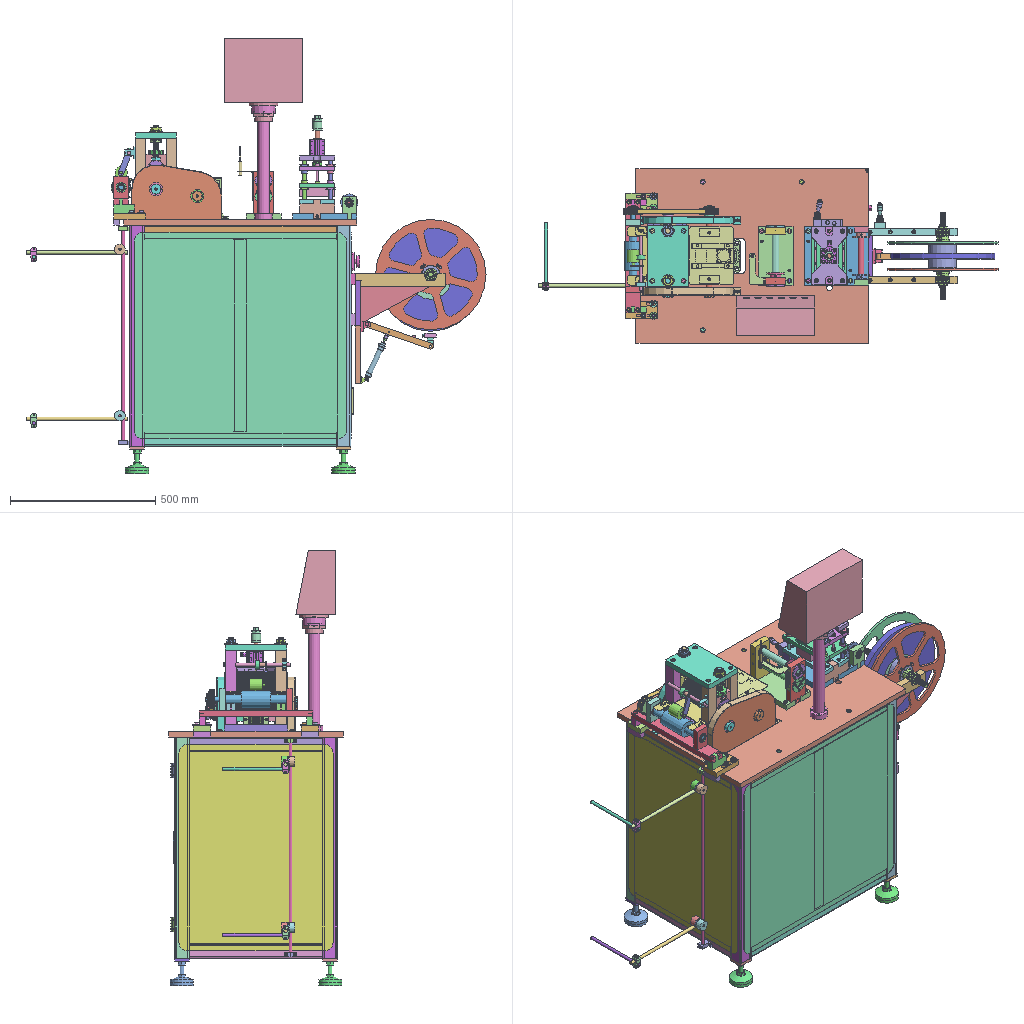Assembly | STEP file | 295 different items | 295 placed | box 1582 x 600 x 1498 mm
Parts list (item | name | quantity | parent item | size | volume):
1 | 1_BODY_id1030_x_t | x1 | in 冲床-300配套压波_x_t | 147.953 x 15 x 147.953 mm | 238621 mm3
2 | 1_BODY_id1118_x_t | x1 | in 冲床-300配套压波_x_t | 148 x 15 x 148 mm | 238417 mm3
3 | 1_BODY_id910_x_t | x1 | in 冲床-300配套压波_x_t | 147.953 x 15 x 147.953 mm | 238621 mm3
4 | 1_BODY_id914_x_t | x1 | in 冲床-300配套压波_x_t | 148 x 15 x 148 mm | 238417 mm3
5 | 2_id534_x_t | x1 | in 冲床-300配套压波_x_t | 270 x 138 x 285.853 mm | 7043394 mm3
6 | 40-1-2-SOLID1_id370_x_t | x1 | in 冲床-300配套压波_x_t | 64 x 12 x 50 mm | 21436 mm3
7 | 40-1-2-SOLID1_id374_x_t | x1 | in 冲床-300配套压波_x_t | 64 x 12 x 50 mm | 21436 mm3
8 | M5X0.8 threaded hole 1_id1086_x_t | x1 | in 冲床-300配套压波_x_t | 158.039 x 110 x 275 mm | 3116162 mm3
9 | Q6.0 _6_ diameter hole 1_id554_x_t | x1 | in 冲床-300配套压波_x_t | 80 x 80 x 390 mm | 160160 mm3
10 | _4H310PA-08_BODY_id414_x_t | x1 | in 冲床-300配套压波_x_t | 40 x 93.887 x 101 mm | 115907 mm3
11 | _4H310PA-08_BODY_id594_x_t | x1 | in 冲床-300配套压波_x_t | 101 x 93.887 x 40 mm | 115907 mm3
12 | - | x1 | in 冲床-300配套压波_x_t | 40 x 37 x 22.5 mm | 5385 mm3
13 | - | x1 | in 冲床-300配套压波_x_t | 40 x 37 x 22.5 mm | 5385 mm3
14 | - | x1 | in 冲床-300配套压波_x_t | 40 x 37 x 22.5 mm | 5385 mm3
15 | - | x1 | in 冲床-300配套压波_x_t | 40 x 37 x 22.5 mm | 5385 mm3
16 | 冲床-300配套压波_id1002_x_t | x1 | in 冲床-300配套压波_x_t | 95 x 103 x 95 mm | 482469 mm3
17 | 冲床-300配套压波_id1006_x_t | x1 | in 冲床-300配套压波_x_t | 380 x 8 x 380 mm | 468890 mm3
18 | 冲床-300配套压波_id1010_x_t | x1 | in 冲床-300配套压波_x_t | 380 x 8 x 380 mm | 468890 mm3
19 | 冲床-300配套压波_id1014_x_t | x1 | in 冲床-300配套压波_x_t | 15 x 540 x 40 mm | 317910 mm3
20 | 冲床-300配套压波_id1018_x_t | x1 | in 冲床-300配套压波_x_t | 1.2 x 530 x 710 mm | 450633 mm3
21 | 冲床-300配套压波_id1022_x_t | x1 | in 冲床-300配套压波_x_t | 1.2 x 530 x 710 mm | 445518 mm3
22 | 冲床-300配套压波_id1026_x_t | x1 | in 冲床-300配套压波_x_t | 90 x 24 x 90 mm | 133155 mm3
23 | 冲床-300配套压波_id102_x_t | x1 | in 冲床-300配套压波_x_t | 13 x 13 x 38 mm | 2405 mm3
24 | 冲床-300配套压波_id1034_x_t | x1 | in 冲床-300配套压波_x_t | 140 x 260 x 24 mm | 727656 mm3
25 | 冲床-300配套压波_id1038_x_t | x1 | in 冲床-300配套压波_x_t | 140 x 38 x 278 mm | 905448 mm3
26 | 冲床-300配套压波_id1042_x_t | x1 | in 冲床-300配套压波_x_t | 140 x 210 x 20 mm | 560119 mm3
27 | 冲床-300配套压波_id1046_x_t | x1 | in 冲床-300配套压波_x_t | 42 x 12 x 42 mm | 8800 mm3
28 | 冲床-300配套压波_id1050_x_t | x1 | in 冲床-300配套压波_x_t | 42 x 12 x 42 mm | 8686 mm3
29 | 冲床-300配套压波_id1054_x_t | x1 | in 冲床-300配套压波_x_t | 42 x 12 x 42 mm | 8686 mm3
30 | 冲床-300配套压波_id1058_x_t | x1 | in 冲床-300配套压波_x_t | 42 x 12 x 42 mm | 8686 mm3
31 | 冲床-300配套压波_id1062_x_t | x1 | in 冲床-300配套压波_x_t | 42 x 12 x 42 mm | 8257 mm3
32 | 冲床-300配套压波_id1066_x_t | x1 | in 冲床-300配套压波_x_t | 42 x 12 x 42 mm | 8257 mm3
33 | 冲床-300配套压波_id106_x_t | x1 | in 冲床-300配套压波_x_t | 13 x 13 x 38 mm | 2405 mm3
34 | 冲床-300配套压波_id1070_x_t | x1 | in 冲床-300配套压波_x_t | 42 x 12 x 42 mm | 8686 mm3
35 | 冲床-300配套压波_id1074_x_t | x1 | in 冲床-300配套压波_x_t | 42 x 12 x 42 mm | 8686 mm3
36 | 冲床-300配套压波_id1078_x_t | x1 | in 冲床-300配套压波_x_t | 28 x 10 x 28 mm | 2984 mm3
37 | 冲床-300配套压波_id1082_x_t | x1 | in 冲床-300配套压波_x_t | 30 x 10 x 30 mm | 3895 mm3
38 | 冲床-300配套压波_id1090_x_t | x1 | in 冲床-300配套压波_x_t | 42.8 x 42.8 x 18 mm | 12253 mm3
39 | 冲床-300配套压波_id1094_x_t | x1 | in 冲床-300配套压波_x_t | 42.8 x 42.8 x 18 mm | 12253 mm3
40 | 冲床-300配套压波_id1098_x_t | x1 | in 冲床-300配套压波_x_t | 86 x 38 x 83 mm | 152873 mm3
41 | 冲床-300配套压波_id10_x_t | x1 | in 冲床-300配套压波_x_t | 13 x 33 x 13 mm | 2154 mm3
42 | 冲床-300配套压波_id1102_x_t | x1 | in 冲床-300配套压波_x_t | 50 x 50 x 14 mm | 18346 mm3
43 | 冲床-300配套压波_id1106_x_t | x1 | in 冲床-300配套压波_x_t | 50 x 50 x 14 mm | 18346 mm3
44 | 冲床-300配套压波_id110_x_t | x1 | in 冲床-300配套压波_x_t | 24 x 24 x 2 mm | 793.943 mm3
45 | 冲床-300配套压波_id1110_x_t | x1 | in 冲床-300配套压波_x_t | 30 x 34.641 x 119.5 mm | 41362 mm3
46 | 冲床-300配套压波_id1114_x_t | x1 | in 冲床-300配套压波_x_t | 30 x 34.641 x 119.5 mm | 41362 mm3
47 | 冲床-300配套压波_id1122_x_t | x1 | in 冲床-300配套压波_x_t | 166 x 112 x 144 mm | 998594 mm3
48 | 冲床-300配套压波_id1126_x_t | x1 | in 冲床-300配套压波_x_t | 40 x 92 x 40 mm | 67089 mm3
49 | 冲床-300配套压波_id1130_x_t | x1 | in 冲床-300配套压波_x_t | 800 x 600 x 20 mm | 9083097 mm3
50 | 冲床-300配套压波_id1134_x_t | x1 | in 冲床-300配套压波_x_t | 50 x 50 x 760 mm | 543703 mm3
51 | 冲床-300配套压波_id1138_x_t | x1 | in 冲床-300配套压波_x_t | 50 x 50 x 760 mm | 543703 mm3
52 | 冲床-300配套压波_id1142_x_t | x1 | in 冲床-300配套压波_x_t | 50 x 50 x 760 mm | 542446 mm3
53 | 冲床-300配套压波_id1146_x_t | x1 | in 冲床-300配套压波_x_t | 50 x 50 x 760 mm | 542446 mm3
54 | 冲床-300配套压波_id114_x_t | x1 | in 冲床-300配套压波_x_t | 13 x 13 x 38 mm | 2405 mm3
55 | 冲床-300配套压波_id1150_x_t | x1 | in 冲床-300配套压波_x_t | 660 x 50 x 50 mm | 470724 mm3
56 | 冲床-300配套压波_id1154_x_t | x1 | in 冲床-300配套压波_x_t | 50 x 460 x 50 mm | 328364 mm3
57 | 冲床-300配套压波_id1158_x_t | x1 | in 冲床-300配套压波_x_t | 50 x 460 x 50 mm | 328364 mm3
58 | 冲床-300配套压波_id1162_x_t | x1 | in 冲床-300配套压波_x_t | 660 x 50 x 50 mm | 470724 mm3
59 | 冲床-300配套压波_id1166_x_t | x1 | in 冲床-300配套压波_x_t | 660 x 50 x 50 mm | 472163 mm3
60 | 冲床-300配套压波_id1170_x_t | x1 | in 冲床-300配套压波_x_t | 50 x 460 x 50 mm | 329083 mm3
61 | 冲床-300配套压波_id1174_x_t | x1 | in 冲床-300配套压波_x_t | 660 x 50 x 50 mm | 472163 mm3
62 | 冲床-300配套压波_id1178_x_t | x1 | in 冲床-300配套压波_x_t | 50 x 460 x 50 mm | 329083 mm3
63 | 冲床-300配套压波_id1182_x_t | x1 | in 冲床-300配套压波_x_t | 50 x 50 x 10 mm | 24142 mm3
64 | 冲床-300配套压波_id118_x_t | x1 | in 冲床-300配套压波_x_t | 18 x 18 x 2 mm | 398.103 mm3
65 | 冲床-300配套压波_id122_x_t | x1 | in 冲床-300配套压波_x_t | 24 x 24 x 2 mm | 793.943 mm3
66 | 冲床-300配套压波_id126_x_t | x1 | in 冲床-300配套压波_x_t | 13 x 13 x 38 mm | 2405 mm3
67 | 冲床-300配套压波_id130_x_t | x1 | in 冲床-300配套压波_x_t | 24 x 24 x 2 mm | 793.943 mm3
68 | 冲床-300配套压波_id134_x_t | x1 | in 冲床-300配套压波_x_t | 13 x 13 x 38 mm | 2405 mm3
69 | 冲床-300配套压波_id138_x_t | x1 | in 冲床-300配套压波_x_t | 16 x 16 x 28 mm | 3059 mm3
70 | 冲床-300配套压波_id142_x_t | x1 | in 冲床-300配套压波_x_t | 16 x 16 x 28 mm | 3059 mm3
71 | 冲床-300配套压波_id146_x_t | x1 | in 冲床-300配套压波_x_t | 16 x 16 x 28 mm | 3059 mm3
72 | 冲床-300配套压波_id14_x_t | x1 | in 冲床-300配套压波_x_t | 16 x 16 x 80 mm | 7143 mm3
73 | 冲床-300配套压波_id150_x_t | x1 | in 冲床-300配套压波_x_t | 16 x 16 x 28 mm | 3059 mm3
74 | 冲床-300配套压波_id154_x_t | x1 | in 冲床-300配套压波_x_t | 10 x 10 x 16 mm | 668.246 mm3
75 | 冲床-300配套压波_id158_x_t | x1 | in 冲床-300配套压波_x_t | 10 x 10 x 16 mm | 668.246 mm3
76 | 冲床-300配套压波_id162_x_t | x1 | in 冲床-300配套压波_x_t | 10 x 10 x 16 mm | 668.246 mm3
77 | 冲床-300配套压波_id166_x_t | x1 | in 冲床-300配套压波_x_t | 11.34 x 11.34 x 10 mm | 408.507 mm3
78 | 冲床-300配套压波_id170_x_t | x1 | in 冲床-300配套压波_x_t | 11.34 x 11.34 x 10 mm | 408.507 mm3
79 | 冲床-300配套压波_id174_x_t | x1 | in 冲床-300配套压波_x_t | 11.34 x 11.34 x 10 mm | 408.507 mm3
80 | 冲床-300配套压波_id178_x_t | x1 | in 冲床-300配套压波_x_t | 50 x 390 x 20 mm | 362265 mm3
81 | 冲床-300配套压波_id182_x_t | x1 | in 冲床-300配套压波_x_t | 70 x 20 x 70 mm | 49405 mm3
82 | 冲床-300配套压波_id186_x_t | x1 | in 冲床-300配套压波_x_t | 20 x 60 x 20 mm | 24000 mm3
83 | 冲床-300配套压波_id18_x_t | x1 | in 冲床-300配套压波_x_t | 16 x 16 x 80 mm | 7143 mm3
84 | 冲床-300配套压波_id190_x_t | x1 | in 冲床-300配套压波_x_t | 110 x 60 x 20 mm | 111155 mm3
85 | 冲床-300配套压波_id194_x_t | x1 | in 冲床-300配套压波_x_t | 11.34 x 11.34 x 10 mm | 408.507 mm3
86 | 冲床-300配套压波_id198_x_t | x1 | in 冲床-300配套压波_x_t | 13 x 13 x 78 mm | 4416 mm3
87 | 冲床-300配套压波_id202_x_t | x1 | in 冲床-300配套压波_x_t | 15.011 x 13 x 7.9 mm | 848.643 mm3
88 | 冲床-300配套压波_id206_x_t | x1 | in 冲床-300配套压波_x_t | 15.011 x 13 x 7.9 mm | 848.643 mm3
89 | 冲床-300配套压波_id210_x_t | x1 | in 冲床-300配套压波_x_t | 13 x 13 x 78 mm | 4416 mm3
90 | 冲床-300配套压波_id214_x_t | x1 | in 冲床-300配套压波_x_t | 13 x 13 x 53 mm | 3159 mm3
91 | 冲床-300配套压波_id218_x_t | x1 | in 冲床-300配套压波_x_t | 13 x 13 x 53 mm | 3159 mm3
92 | 冲床-300配套压波_id222_x_t | x1 | in 冲床-300配套压波_x_t | 13 x 13 x 53 mm | 3159 mm3
93 | 冲床-300配套压波_id226_x_t | x1 | in 冲床-300配套压波_x_t | 13 x 13 x 53 mm | 3159 mm3
94 | 冲床-300配套压波_id22_x_t | x1 | in 冲床-300配套压波_x_t | 16 x 16 x 80 mm | 7143 mm3
95 | 冲床-300配套压波_id230_x_t | x1 | in 冲床-300配套压波_x_t | 16 x 16 x 30 mm | 3216 mm3
96 | 冲床-300配套压波_id234_x_t | x1 | in 冲床-300配套压波_x_t | 16 x 16 x 30 mm | 3216 mm3
97 | 冲床-300配套压波_id238_x_t | x1 | in 冲床-300配套压波_x_t | 16 x 16 x 30 mm | 3216 mm3
98 | 冲床-300配套压波_id242_x_t | x1 | in 冲床-300配套压波_x_t | 16 x 16 x 30 mm | 3216 mm3
99 | 冲床-300配套压波_id246_x_t | x1 | in 冲床-300配套压波_x_t | 16 x 16 x 30 mm | 3216 mm3
100 | 冲床-300配套压波_id250_x_t | x1 | in 冲床-300配套压波_x_t | 16 x 16 x 30 mm | 3216 mm3
101 | 冲床-300配套压波_id254_x_t | x1 | in 冲床-300配套压波_x_t | 16 x 16 x 30 mm | 3216 mm3
102 | 冲床-300配套压波_id258_x_t | x1 | in 冲床-300配套压波_x_t | 16 x 16 x 30 mm | 3216 mm3
103 | 冲床-300配套压波_id262_x_t | x1 | in 冲床-300配套压波_x_t | 50 x 20 x 95.5 mm | 62578 mm3
104 | 冲床-300配套压波_id266_x_t | x1 | in 冲床-300配套压波_x_t | 35 x 10 x 35 mm | 4991 mm3
105 | 冲床-300配套压波_id26_x_t | x1 | in 冲床-300配套压波_x_t | 16 x 16 x 80 mm | 7143 mm3
106 | 冲床-300配套压波_id270_x_t | x1 | in 冲床-300配套压波_x_t | 35 x 10 x 35 mm | 4991 mm3
107 | 冲床-300配套压波_id274_x_t | x1 | in 冲床-300配套压波_x_t | 327.52 x 16 x 95.437 mm | 33845 mm3
108 | 冲床-300配套压波_id278_x_t | x1 | in 冲床-300配套压波_x_t | 38 x 14 x 42 mm | 10740 mm3
109 | 冲床-300配套压波_id282_x_t | x1 | in 冲床-300配套压波_x_t | 12 x 188 x 12 mm | 21262 mm3
110 | 冲床-300配套压波_id286_x_t | x1 | in 冲床-300配套压波_x_t | 41.5 x 59 x 41.5 mm | 60695 mm3
111 | 冲床-300配套压波_id290_x_t | x1 | in 冲床-300配套压波_x_t | 47 x 5 x 88.25 mm | 7952 mm3
112 | 冲床-300配套压波_id294_x_t | x1 | in 冲床-300配套压波_x_t | 15 x 20 x 15 mm | 3534 mm3
113 | 冲床-300配套压波_id298_x_t | x1 | in 冲床-300配套压波_x_t | 30 x 15 x 30 mm | 10603 mm3
114 | 冲床-300配套压波_id302_x_t | x1 | in 冲床-300配套压波_x_t | 20 x 60 x 20 mm | 24000 mm3
115 | 冲床-300配套压波_id306_x_t | x1 | in 冲床-300配套压波_x_t | 28 x 85.6 x 90 mm | 124096 mm3
116 | 冲床-300配套压波_id30_x_t | x1 | in 冲床-300配套压波_x_t | 16 x 16 x 80 mm | 7143 mm3
117 | 冲床-300配套压波_id310_x_t | x1 | in 冲床-300配套压波_x_t | 60 x 297 x 60 mm | 378054 mm3
118 | 冲床-300配套压波_id314_x_t | x1 | in 冲床-300配套压波_x_t | 67 x 28.5 x 67 mm | 59308 mm3
119 | 冲床-300配套压波_id318_x_t | x1 | in 冲床-300配套压波_x_t | 67 x 28.5 x 67 mm | 58410 mm3
120 | 冲床-300配套压波_id322_x_t | x1 | in 冲床-300配套压波_x_t | 35 x 10 x 35 mm | 4991 mm3
121 | 冲床-300配套压波_id326_x_t | x1 | in 冲床-300配套压波_x_t | 35 x 10 x 35 mm | 4991 mm3
122 | 冲床-300配套压波_id330_x_t | x1 | in 冲床-300配套压波_x_t | 50 x 20 x 95.5 mm | 62578 mm3
123 | 冲床-300配套压波_id334_x_t | x1 | in 冲床-300配套压波_x_t | 70 x 20 x 70 mm | 49405 mm3
124 | 冲床-300配套压波_id338_x_t | x1 | in 冲床-300配套压波_x_t | 110 x 60 x 20 mm | 111155 mm3
125 | 冲床-300配套压波_id342_x_t | x1 | in 冲床-300配套压波_x_t | 300 x 15 x 655 mm | 275574 mm3
126 | 冲床-300配套压波_id346_x_t | x1 | in 冲床-300配套压波_x_t | 70 x 24 x 163 mm | 181383 mm3
127 | 冲床-300配套压波_id34_x_t | x1 | in 冲床-300配套压波_x_t | 16 x 16 x 80 mm | 7143 mm3
128 | 冲床-300配套压波_id350_x_t | x1 | in 冲床-300配套压波_x_t | 59 x 5 x 54 mm | 8662 mm3
129 | 冲床-300配套压波_id354_x_t | x1 | in 冲床-300配套压波_x_t | 59 x 5 x 54 mm | 8662 mm3
130 | 冲床-300配套压波_id358_x_t | x1 | in 冲床-300配套压波_x_t | 70 x 24 x 163 mm | 181383 mm3
131 | 冲床-300配套压波_id362_x_t | x1 | in 冲床-300配套压波_x_t | 59 x 5 x 54 mm | 8662 mm3
132 | 冲床-300配套压波_id366_x_t | x1 | in 冲床-300配套压波_x_t | 59 x 5 x 59 mm | 9584 mm3
133 | 冲床-300配套压波_id378_x_t | x1 | in 冲床-300配套压波_x_t | 80 x 1.2 x 80 mm | 3840 mm3
134 | 冲床-300配套压波_id38_x_t | x1 | in 冲床-300配套压波_x_t | 10 x 10 x 18 mm | 724.794 mm3
135 | 冲床-300配套压波_id398_x_t | x1 | in 冲床-300配套压波_x_t | 80 x 1.2 x 80 mm | 3840 mm3
136 | 冲床-300配套压波_id402_x_t | x1 | in 冲床-300配套压波_x_t | 80 x 1.2 x 80 mm | 3840 mm3
137 | 冲床-300配套压波_id406_x_t | x1 | in 冲床-300配套压波_x_t | 80 x 1.2 x 80 mm | 3840 mm3
138 | 冲床-300配套压波_id410_x_t | x1 | in 冲床-300配套压波_x_t | 307 x 1.2 x 186.5 mm | 57177 mm3
139 | 冲床-300配套压波_id418_x_t | x1 | in 冲床-300配套压波_x_t | 64 x 60 x 60 mm | 90346 mm3
140 | 冲床-300配套压波_id422_x_t | x1 | in 冲床-300配套压波_x_t | 50 x 12.7 x 49.8 mm | 17221 mm3
141 | 冲床-300配套压波_id426_x_t | x1 | in 冲床-300配套压波_x_t | 50 x 12.7 x 49.8 mm | 17221 mm3
142 | 冲床-300配套压波_id42_x_t | x1 | in 冲床-300配套压波_x_t | 10 x 10 x 18 mm | 724.794 mm3
143 | 冲床-300配套压波_id430_x_t | x1 | in 冲床-300配套压波_x_t | 25 x 270 x 25 mm | 98996 mm3
144 | 冲床-300配套压波_id434_x_t | x1 | in 冲床-300配套压波_x_t | 42 x 12 x 42 mm | 8686 mm3
145 | 冲床-300配套压波_id438_x_t | x1 | in 冲床-300配套压波_x_t | 42 x 12 x 42 mm | 8686 mm3
146 | 冲床-300配套压波_id442_x_t | x1 | in 冲床-300配套压波_x_t | 59 x 5 x 59 mm | 9584 mm3
147 | 冲床-300配套压波_id446_x_t | x1 | in 冲床-300配套压波_x_t | 42 x 12 x 42 mm | 8686 mm3
148 | 冲床-300配套压波_id450_x_t | x1 | in 冲床-300配套压波_x_t | 42 x 12 x 42 mm | 8686 mm3
149 | 冲床-300配套压波_id454_x_t | x1 | in 冲床-300配套压波_x_t | 36 x 20.5 x 36 mm | 15877 mm3
150 | 冲床-300配套压波_id458_x_t | x1 | in 冲床-300配套压波_x_t | 36 x 5 x 36 mm | 4806 mm3
151 | 冲床-300配套压波_id462_x_t | x1 | in 冲床-300配套压波_x_t | 36 x 20.5 x 36 mm | 17065 mm3
152 | 冲床-300配套压波_id466_x_t | x1 | in 冲床-300配套压波_x_t | 12 x 230 x 12 mm | 26012 mm3
153 | 冲床-300配套压波_id46_x_t | x1 | in 冲床-300配套压波_x_t | 16 x 16 x 30 mm | 3216 mm3
154 | 冲床-300配套压波_id470_x_t | x1 | in 冲床-300配套压波_x_t | 21 x 21 x 50 mm | 11568 mm3
155 | 冲床-300配套压波_id474_x_t | x1 | in 冲床-300配套压波_x_t | 350 x 12 x 12 mm | 39584 mm3
156 | 冲床-300配套压波_id478_x_t | x1 | in 冲床-300配套压波_x_t | 36 x 5 x 36 mm | 4806 mm3
157 | 冲床-300配套压波_id482_x_t | x1 | in 冲床-300配套压波_x_t | 36 x 20.5 x 36 mm | 15877 mm3
158 | 冲床-300配套压波_id486_x_t | x1 | in 冲床-300配套压波_x_t | 21 x 21 x 50 mm | 11568 mm3
159 | 冲床-300配套压波_id490_x_t | x1 | in 冲床-300配套压波_x_t | 12 x 230 x 12 mm | 26012 mm3
160 | 冲床-300配套压波_id494_x_t | x1 | in 冲床-300配套压波_x_t | 350 x 12 x 12 mm | 39584 mm3
161 | 冲床-300配套压波_id498_x_t | x1 | in 冲床-300配套压波_x_t | 36 x 20.5 x 36 mm | 17065 mm3
162 | 冲床-300配套压波_id502_x_t | x1 | in 冲床-300配套压波_x_t | 12 x 12 x 750 mm | 84823 mm3
163 | 冲床-300配套压波_id506_x_t | x1 | in 冲床-300配套压波_x_t | 38 x 42 x 14 mm | 10740 mm3
164 | 冲床-300配套压波_id50_x_t | x1 | in 冲床-300配套压波_x_t | 16 x 16 x 30 mm | 3216 mm3
165 | 冲床-300配套压波_id510_x_t | x1 | in 冲床-300配套压波_x_t | 38 x 42 x 14 mm | 10740 mm3
166 | 冲床-300配套压波_id514_x_t | x1 | in 冲床-300配套压波_x_t | 307 x 1.5 x 186.5 mm | 71471 mm3
167 | 冲床-300配套压波_id518_x_t | x1 | in 冲床-300配套压波_x_t | 730 x 1.2 x 710 mm | 621033 mm3
168 | 冲床-300配套压波_id522_x_t | x1 | in 冲床-300配套压波_x_t | 69 x 21 x 119 mm | 44051 mm3
169 | 冲床-300配套压波_id526_x_t | x1 | in 冲床-300配套压波_x_t | 300 x 15 x 655 mm | 275574 mm3
170 | 冲床-300配套压波_id530_x_t | x1 | in 冲床-300配套压波_x_t | 69 x 21 x 119 mm | 44051 mm3
171 | 冲床-300配套压波_id538_x_t | x1 | in 冲床-300配套压波_x_t | 30 x 30 x 30 mm | 12788 mm3
172 | 冲床-300配套压波_id542_x_t | x1 | in 冲床-300配套压波_x_t | 120 x 30 x 65 mm | 132651 mm3
173 | 冲床-300配套压波_id546_x_t | x1 | in 冲床-300配套压波_x_t | 360 x 25 x 188 mm | 23610 mm3
174 | 冲床-300配套压波_id54_x_t | x1 | in 冲床-300配套压波_x_t | 16 x 16 x 30 mm | 3216 mm3
175 | 冲床-300配套压波_id550_x_t | x1 | in 冲床-300配套压波_x_t | 360 x 25 x 187.7 mm | 18888 mm3
176 | 冲床-300配套压波_id558_x_t | x1 | in 冲床-300配套压波_x_t | 55 x 109 x 100 mm | 9589 mm3
177 | 冲床-300配套压波_id562_x_t | x1 | in 冲床-300配套压波_x_t | 35 x 270 x 35 mm | 104906 mm3
178 | 冲床-300配套压波_id566_x_t | x1 | in 冲床-300配套压波_x_t | 69.832 x 130 x 69.818 mm | 396551 mm3
179 | 冲床-300配套压波_id570_x_t | x1 | in 冲床-300配套压波_x_t | 69.832 x 130 x 69.818 mm | 396551 mm3
180 | 冲床-300配套压波_id574_x_t | x1 | in 冲床-300配套压波_x_t | 35 x 210 x 35 mm | 89544 mm3
181 | 冲床-300配套压波_id578_x_t | x1 | in 冲床-300配套压波_x_t | 118 x 200 x 2 mm | 26939 mm3
182 | 冲床-300配套压波_id582_x_t | x1 | in 冲床-300配套压波_x_t | 40 x 30 x 80 mm | 9315 mm3
183 | 冲床-300配套压波_id586_x_t | x1 | in 冲床-300配套压波_x_t | 60 x 16 x 60 mm | 19955 mm3
184 | 冲床-300配套压波_id58_x_t | x1 | in 冲床-300配套压波_x_t | 16 x 16 x 30 mm | 3216 mm3
185 | 冲床-300配套压波_id590_x_t | x1 | in 冲床-300配套压波_x_t | 40 x 30 x 80 mm | 9315 mm3
186 | 冲床-300配套压波_id598_x_t | x1 | in 冲床-300配套压波_x_t | 35 x 15 x 35 mm | 11277 mm3
187 | 冲床-300配套压波_id602_x_t | x1 | in 冲床-300配套压波_x_t | 35 x 45 x 35 mm | 14863 mm3
188 | 冲床-300配套压波_id606_x_t | x1 | in 冲床-300配套压波_x_t | 35 x 15 x 35 mm | 11277 mm3
189 | 冲床-300配套压波_id610_x_t | x1 | in 冲床-300配套压波_x_t | 59 x 19 x 59 mm | 24068 mm3
190 | 冲床-300配套压波_id614_x_t | x1 | in 冲床-300配套压波_x_t | 80 x 80 x 145 mm | 156529 mm3
191 | 冲床-300配套压波_id618_x_t | x1 | in 冲床-300配套压波_x_t | 80 x 80 x 145 mm | 156529 mm3
192 | 冲床-300配套压波_id622_x_t | x1 | in 冲床-300配套压波_x_t | 80 x 80 x 145 mm | 156529 mm3
193 | 冲床-300配套压波_id626_x_t | x1 | in 冲床-300配套压波_x_t | 59 x 19 x 59 mm | 24068 mm3
194 | 冲床-300配套压波_id62_x_t | x1 | in 冲床-300配套压波_x_t | 10 x 10 x 40 mm | 2825 mm3
195 | 冲床-300配套压波_id630_x_t | x1 | in 冲床-300配套压波_x_t | 59 x 10.5 x 59 mm | 15635 mm3
196 | 冲床-300配套压波_id634_x_t | x1 | in 冲床-300配套压波_x_t | 35 x 15 x 35 mm | 11277 mm3
197 | 冲床-300配套压波_id638_x_t | x1 | in 冲床-300配套压波_x_t | 40 x 40 x 15 mm | 12585 mm3
198 | 冲床-300配套压波_id642_x_t | x1 | in 冲床-300配套压波_x_t | 40 x 40 x 15 mm | 11990 mm3
199 | 冲床-300配套压波_id646_x_t | x1 | in 冲床-300配套压波_x_t | 21.939 x 19 x 8 mm | 1254 mm3
200 | 冲床-300配套压波_id650_x_t | x1 | in 冲床-300配套压波_x_t | 16 x 16 x 173 mm | 33408 mm3
201 | 冲床-300配套压波_id654_x_t | x1 | in 冲床-300配套压波_x_t | 32 x 32 x 49 mm | 24682 mm3
202 | 冲床-300配套压波_id658_x_t | x1 | in 冲床-300配套压波_x_t | 52 x 78.5 x 62 mm | 126895 mm3
203 | 冲床-300配套压波_id662_x_t | x1 | in 冲床-300配套压波_x_t | 86 x 38 x 83 mm | 152874 mm3
204 | 冲床-300配套压波_id666_x_t | x1 | in 冲床-300配套压波_x_t | 74.68 x 22 x 134.608 mm | 35462 mm3
205 | 冲床-300配套压波_id66_x_t | x1 | in 冲床-300配套压波_x_t | 10 x 10 x 40 mm | 2825 mm3
206 | 冲床-300配套压波_id670_x_t | x1 | in 冲床-300配套压波_x_t | 32 x 52 x 52 mm | 31697 mm3
207 | 冲床-300配套压波_id674_x_t | x1 | in 冲床-300配套压波_x_t | 65.907 x 10 x 131.805 mm | 4315 mm3
208 | 冲床-300配套压波_id678_x_t | x1 | in 冲床-300配套压波_x_t | 22.859 x 12 x 31.872 mm | 2285 mm3
209 | 冲床-300配套压波_id682_x_t | x1 | in 冲床-300配套压波_x_t | 237.457 x 20 x 94.916 mm | 85651 mm3
210 | 冲床-300配套压波_id686_x_t | x1 | in 冲床-300配套压波_x_t | 20.046 x 30 x 40.015 mm | 10464 mm3
211 | 冲床-300配套压波_id690_x_t | x1 | in 冲床-300配套压波_x_t | 40.015 x 40 x 15.054 mm | 21445 mm3
212 | 冲床-300配套压波_id694_x_t | x1 | in 冲床-300配套压波_x_t | 25.1 x 40 x 23 mm | 2627 mm3
213 | 冲床-300配套压波_id698_x_t | x1 | in 冲床-300配套压波_x_t | 60 x 16 x 60 mm | 19587 mm3
214 | 冲床-300配套压波_id6_x_t | x1 | in 冲床-300配套压波_x_t | 13 x 33 x 13 mm | 2154 mm3
215 | 冲床-300配套压波_id702_x_t | x1 | in 冲床-300配套压波_x_t | 60 x 16 x 60 mm | 19587 mm3
216 | 冲床-300配套压波_id706_x_t | x1 | in 冲床-300配套压波_x_t | 80 x 80 x 145 mm | 156529 mm3
217 | 冲床-300配套压波_id70_x_t | x1 | in 冲床-300配套压波_x_t | 10 x 10 x 40 mm | 2825 mm3
218 | 冲床-300配套压波_id710_x_t | x1 | in 冲床-300配套压波_x_t | 59 x 5 x 54 mm | 8662 mm3
219 | 冲床-300配套压波_id714_x_t | x1 | in 冲床-300配套压波_x_t | 10 x 10 x 100 mm | 4206 mm3
220 | 冲床-300配套压波_id718_x_t | x1 | in 冲床-300配套压波_x_t | 16.012 x 10 x 10.009 mm | 668.246 mm3
221 | 冲床-300配套压波_id722_x_t | x1 | in 冲床-300配套压波_x_t | 12.775 x 10 x 17.733 mm | 668.246 mm3
222 | 冲床-300配套压波_id726_x_t | x1 | in 冲床-300配套压波_x_t | 50 x 460 x 50 mm | 329083 mm3
223 | 冲床-300配套压波_id730_x_t | x1 | in 冲床-300配套压波_x_t | 360 x 20 x 360 mm | 1727876 mm3
224 | 冲床-300配套压波_id734_x_t | x1 | in 冲床-300配套压波_x_t | 20 x 60 x 240 mm | 277564 mm3
225 | 冲床-300配套压波_id738_x_t | x1 | in 冲床-300配套压波_x_t | 140 x 20 x 140 mm | 166112 mm3
226 | 冲床-300配套压波_id742_x_t | x1 | in 冲床-300配套压波_x_t | 32 x 10 x 32 mm | 4744 mm3
227 | 冲床-300配套压波_id746_x_t | x1 | in 冲床-300配套压波_x_t | 32 x 10 x 32 mm | 4744 mm3
228 | 冲床-300配套压波_id74_x_t | x1 | in 冲床-300配套压波_x_t | 10 x 10 x 40 mm | 2825 mm3
229 | 冲床-300配套压波_id750_x_t | x1 | in 冲床-300配套压波_x_t | 32 x 10 x 32 mm | 4744 mm3
230 | 冲床-300配套压波_id754_x_t | x1 | in 冲床-300配套压波_x_t | 20 x 200 x 20 mm | 54754 mm3
231 | 冲床-300配套压波_id758_x_t | x1 | in 冲床-300配套压波_x_t | 32 x 10 x 32 mm | 4744 mm3
232 | 冲床-300配套压波_id762_x_t | x1 | in 冲床-300配套压波_x_t | 120 x 200 x 15 mm | 229658 mm3
233 | 冲床-300配套压波_id766_x_t | x1 | in 冲床-300配套压波_x_t | 50 x 460 x 50 mm | 329083 mm3
234 | 冲床-300配套压波_id770_x_t | x1 | in 冲床-300配套压波_x_t | 12 x 12 x 160 mm | 17294 mm3
235 | 冲床-300配套压波_id774_x_t | x1 | in 冲床-300配套压波_x_t | 12 x 12 x 160 mm | 17294 mm3
236 | 冲床-300配套压波_id778_x_t | x1 | in 冲床-300配套压波_x_t | 32 x 32 x 30 mm | 10494 mm3
237 | 冲床-300配套压波_id782_x_t | x1 | in 冲床-300配套压波_x_t | 32 x 32 x 30 mm | 10494 mm3
238 | 冲床-300配套压波_id786_x_t | x1 | in 冲床-300配套压波_x_t | 32 x 32 x 30 mm | 10494 mm3
239 | 冲床-300配套压波_id78_x_t | x1 | in 冲床-300配套压波_x_t | 10 x 10 x 40 mm | 2825 mm3
240 | 冲床-300配套压波_id790_x_t | x1 | in 冲床-300配套压波_x_t | 32 x 32 x 30 mm | 10494 mm3
241 | 冲床-300配套压波_id794_x_t | x1 | in 冲床-300配套压波_x_t | 32 x 32 x 30 mm | 10494 mm3
242 | 冲床-300配套压波_id798_x_t | x1 | in 冲床-300配套压波_x_t | 32 x 32 x 30 mm | 10494 mm3
243 | 冲床-300配套压波_id802_x_t | x1 | in 冲床-300配套压波_x_t | 32 x 32 x 30 mm | 10494 mm3
244 | 冲床-300配套压波_id806_x_t | x1 | in 冲床-300配套压波_x_t | 32 x 32 x 30 mm | 10494 mm3
245 | 冲床-300配套压波_id810_x_t | x1 | in 冲床-300配套压波_x_t | 120 x 200 x 20 mm | 424966 mm3
246 | 冲床-300配套压波_id814_x_t | x1 | in 冲床-300配套压波_x_t | 42 x 12 x 42 mm | 8804 mm3
247 | 冲床-300配套压波_id818_x_t | x1 | in 冲床-300配套压波_x_t | 42 x 12 x 42 mm | 8804 mm3
248 | 冲床-300配套压波_id822_x_t | x1 | in 冲床-300配套压波_x_t | 25 x 200 x 25 mm | 89339 mm3
249 | 冲床-300配套压波_id826_x_t | x1 | in 冲床-300配套压波_x_t | 42 x 12 x 42 mm | 8804 mm3
250 | 冲床-300配套压波_id82_x_t | x1 | in 冲床-300配套压波_x_t | 10 x 10 x 40 mm | 2825 mm3
251 | 冲床-300配套压波_id830_x_t | x1 | in 冲床-300配套压波_x_t | 42 x 12 x 42 mm | 8804 mm3
252 | 冲床-300配套压波_id834_x_t | x1 | in 冲床-300配套压波_x_t | 42 x 12 x 42 mm | 8804 mm3
253 | 冲床-300配套压波_id838_x_t | x1 | in 冲床-300配套压波_x_t | 42 x 12 x 42 mm | 8804 mm3
254 | 冲床-300配套压波_id842_x_t | x1 | in 冲床-300配套压波_x_t | 25 x 200 x 25 mm | 89339 mm3
255 | 冲床-300配套压波_id846_x_t | x1 | in 冲床-300配套压波_x_t | 42 x 12 x 42 mm | 8804 mm3
256 | 冲床-300配套压波_id850_x_t | x1 | in 冲床-300配套压波_x_t | 42 x 12 x 42 mm | 8804 mm3
257 | 冲床-300配套压波_id854_x_t | x1 | in 冲床-300配套压波_x_t | 120 x 200 x 15 mm | 324088 mm3
258 | 冲床-300配套压波_id858_x_t | x1 | in 冲床-300配套压波_x_t | 120 x 70 x 30 mm | 248979 mm3
259 | 冲床-300配套压波_id862_x_t | x1 | in 冲床-300配套压波_x_t | 12 x 12 x 160 mm | 17294 mm3
260 | 冲床-300配套压波_id866_x_t | x1 | in 冲床-300配套压波_x_t | 12 x 12 x 160 mm | 17294 mm3
261 | 冲床-300配套压波_id86_x_t | x1 | in 冲床-300配套压波_x_t | 10 x 10 x 16 mm | 668.246 mm3
262 | 冲床-300配套压波_id870_x_t | x1 | in 冲床-300配套压波_x_t | 120 x 30 x 65 mm | 132651 mm3
263 | 冲床-300配套压波_id874_x_t | x1 | in 冲床-300配套压波_x_t | 120 x 200 x 15 mm | 311095 mm3
264 | 冲床-300配套压波_id878_x_t | x1 | in 冲床-300配套压波_x_t | 120 x 200 x 15 mm | 240910 mm3
265 | 冲床-300配套压波_id882_x_t | x1 | in 冲床-300配套压波_x_t | 204.24 x 200 x 10.652 mm | 74480 mm3
266 | 冲床-300配套压波_id886_x_t | x1 | in 冲床-300配套压波_x_t | 220 x 200 x 20 mm | 814165 mm3
267 | 冲床-300配套压波_id890_x_t | x1 | in 冲床-300配套压波_x_t | 50 x 20 x 79 mm | 49384 mm3
268 | 冲床-300配套压波_id894_x_t | x1 | in 冲床-300配套压波_x_t | 50 x 20 x 79 mm | 49384 mm3
269 | 冲床-300配套压波_id898_x_t | x1 | in 冲床-300配套压波_x_t | 50 x 50 x 10 mm | 24142 mm3
270 | 冲床-300配套压波_id902_x_t | x1 | in 冲床-300配套压波_x_t | 50 x 50 x 10 mm | 24142 mm3
271 | 冲床-300配套压波_id906_x_t | x1 | in 冲床-300配套压波_x_t | 50 x 50 x 10 mm | 24142 mm3
272 | 冲床-300配套压波_id90_x_t | x1 | in 冲床-300配套压波_x_t | 13 x 13 x 38 mm | 2405 mm3
273 | 冲床-300配套压波_id918_x_t | x1 | in 冲床-300配套压波_x_t | 140 x 29 x 142 mm | 300034 mm3
274 | 冲床-300配套压波_id922_x_t | x1 | in 冲床-300配套压波_x_t | 16 x 16 x 50 mm | 4786 mm3
275 | 冲床-300配套压波_id926_x_t | x1 | in 冲床-300配套压波_x_t | 20 x 20 x 3 mm | 657.378 mm3
276 | 冲床-300配套压波_id930_x_t | x1 | in 冲床-300配套压波_x_t | 16 x 16 x 50 mm | 4786 mm3
277 | 冲床-300配套压波_id934_x_t | x1 | in 冲床-300配套压波_x_t | 20 x 20 x 3 mm | 657.378 mm3
278 | 冲床-300配套压波_id938_x_t | x1 | in 冲床-300配套压波_x_t | 16 x 16 x 50 mm | 4786 mm3
279 | 冲床-300配套压波_id942_x_t | x1 | in 冲床-300配套压波_x_t | 140 x 29 x 142 mm | 284024 mm3
280 | 冲床-300配套压波_id946_x_t | x1 | in 冲床-300配套压波_x_t | 20 x 20 x 3 mm | 657.378 mm3
281 | 冲床-300配套压波_id94_x_t | x1 | in 冲床-300配套压波_x_t | 18 x 18 x 2 mm | 398.103 mm3
282 | 冲床-300配套压波_id950_x_t | x1 | in 冲床-300配套压波_x_t | 16 x 16 x 50 mm | 4786 mm3
283 | 冲床-300配套压波_id954_x_t | x1 | in 冲床-300配套压波_x_t | 20 x 20 x 3 mm | 657.378 mm3
284 | 冲床-300配套压波_id958_x_t | x1 | in 冲床-300配套压波_x_t | 90 x 24 x 90 mm | 133155 mm3
285 | 冲床-300配套压波_id962_x_t | x1 | in 冲床-300配套压波_x_t | 140 x 38 x 278 mm | 905448 mm3
286 | 冲床-300配套压波_id966_x_t | x1 | in 冲床-300配套压波_x_t | 50 x 50 x 660 mm | 472163 mm3
287 | 冲床-300配套压波_id970_x_t | x1 | in 冲床-300配套压波_x_t | 50 x 50 x 660 mm | 472163 mm3
288 | 冲床-300配套压波_id974_x_t | x1 | in 冲床-300配套压波_x_t | 237.857 x 15 x 120 mm | 224363 mm3
289 | 冲床-300配套压波_id978_x_t | x1 | in 冲床-300配套压波_x_t | 237.857 x 15 x 120 mm | 223740 mm3
290 | 冲床-300配套压波_id982_x_t | x1 | in 冲床-300配套压波_x_t | 20 x 190 x 180 mm | 579376 mm3
291 | 冲床-300配套压波_id986_x_t | x1 | in 冲床-300配套压波_x_t | 310 x 25 x 45 mm | 301509 mm3
292 | 冲床-300配套压波_id98_x_t | x1 | in 冲床-300配套压波_x_t | 24 x 24 x 2 mm | 793.943 mm3
293 | 冲床-300配套压波_id990_x_t | x1 | in 冲床-300配套压波_x_t | 310 x 25 x 45 mm | 301509 mm3
294 | 冲床-300配套压波_id994_x_t | x1 | in 冲床-300配套压波_x_t | 15 x 540 x 40 mm | 319568 mm3
295 | 冲床-300配套压波_id998_x_t | x1 | in 冲床-300配套压波_x_t | - | -